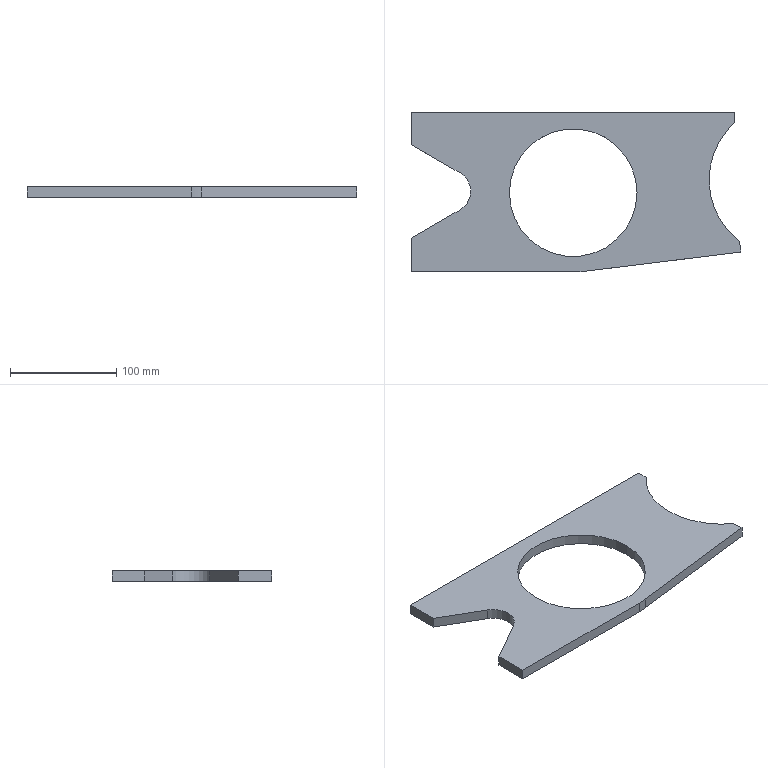Part | SolidWorks | features Extrusion 1 | 1 solid | 17 faces | box 309.8 x 150 x 10 mm | volume 282199 mm3 | plane 11 | cylinder 6 | commonest cylinder face diameters 120 x2 144.6 x2 40 x1 150 x1
STEP:
#1=CARTESIAN_POINT('',(-260.,-12.,10.));
#2=VERTEX_POINT('',#1);
#3=CARTESIAN_POINT('',(-140.,-12.,10.));
#4=VERTEX_POINT('',#3);
#5=CARTESIAN_POINT('',(-200.,-12.,10.));
#6=DIRECTION('',(0.,0.,1.));
#7=DIRECTION('',(1.,0.,0.));
#8=AXIS2_PLACEMENT_3D('',#5,#6,#7);
#9=CIRCLE('',#8,60.);
#10=EDGE_CURVE('',#2,#4,#9,.T.);
#11=ORIENTED_EDGE('',*,*,#10,.T.);
#12=CARTESIAN_POINT('',(-140.,-12.,0.));
#13=VERTEX_POINT('',#12);
#14=CARTESIAN_POINT('',(-140.,-12.,10.));
#15=DIRECTION('',(0.,0.,-1.));
#16=VECTOR('',#15,1000.);
#17=LINE('',#14,#16);
#18=EDGE_CURVE('',#4,#13,#17,.T.);
#19=ORIENTED_EDGE('',*,*,#18,.T.);
#20=CARTESIAN_POINT('',(-260.,-12.,0.));
#21=VERTEX_POINT('',#20);
#22=CARTESIAN_POINT('',(-200.,-12.,0.));
#23=DIRECTION('',(0.,0.,1.));
#24=DIRECTION('',(1.,0.,0.));
#25=AXIS2_PLACEMENT_3D('',#22,#23,#24);
#26=CIRCLE('',#25,60.);
#27=EDGE_CURVE('',#21,#13,#26,.T.);
#28=ORIENTED_EDGE('',*,*,#27,.F.);
#29=CARTESIAN_POINT('',(-260.,-12.,10.));
#30=DIRECTION('',(0.,0.,-1.));
#31=VECTOR('',#30,1000.);
#32=LINE('',#29,#31);
#33=EDGE_CURVE('',#2,#21,#32,.T.);
#34=ORIENTED_EDGE('',*,*,#33,.F.);
#35=EDGE_LOOP('',(#11,#19,#28,#34));
#36=FACE_OUTER_BOUND('',#35,.T.);
#37=CARTESIAN_POINT('',(-200.,-12.,10.));
#38=DIRECTION('',(0.,0.,-1.));
#39=DIRECTION('',(-1.,0.,0.));
#40=AXIS2_PLACEMENT_3D('',#37,#38,#39);
#41=CYLINDRICAL_SURFACE('',#40,60.);
#42=ADVANCED_FACE('',(#36),#41,.F.);
#43=CARTESIAN_POINT('',(-72.3,0.,10.));
#44=VERTEX_POINT('',#43);
#45=CARTESIAN_POINT('',(-48.3,53.8,10.));
#46=VERTEX_POINT('',#45);
#47=CARTESIAN_POINT('',(0.,0.,10.));
#48=DIRECTION('',(0.,0.,-1.));
#49=DIRECTION('',(1.,0.,0.));
#50=AXIS2_PLACEMENT_3D('',#47,#48,#49);
#51=CIRCLE('',#50,72.3);
#52=EDGE_CURVE('',#44,#46,#51,.T.);
#53=ORIENTED_EDGE('',*,*,#52,.F.);
#54=CARTESIAN_POINT('',(-72.3,0.,0.));
#55=VERTEX_POINT('',#54);
#56=CARTESIAN_POINT('',(-72.3,0.,10.));
#57=DIRECTION('',(0.,0.,-1.));
#58=VECTOR('',#57,1000.);
#59=LINE('',#56,#58);
#60=EDGE_CURVE('',#44,#55,#59,.T.);
#61=ORIENTED_EDGE('',*,*,#60,.T.);
#62=CARTESIAN_POINT('',(-48.3,53.8,0.));
#63=VERTEX_POINT('',#62);
#64=CARTESIAN_POINT('',(0.,0.,0.));
#65=DIRECTION('',(0.,0.,-1.));
#66=DIRECTION('',(1.,0.,0.));
#67=AXIS2_PLACEMENT_3D('',#64,#65,#66);
#68=CIRCLE('',#67,72.3);
#69=EDGE_CURVE('',#55,#63,#68,.T.);
#70=ORIENTED_EDGE('',*,*,#69,.T.);
#71=CARTESIAN_POINT('',(-48.3,53.8,10.));
#72=DIRECTION('',(0.,0.,-1.));
#73=VECTOR('',#72,1000.);
#74=LINE('',#71,#73);
#75=EDGE_CURVE('',#46,#63,#74,.T.);
#76=ORIENTED_EDGE('',*,*,#75,.F.);
#77=EDGE_LOOP('',(#53,#61,#70,#76));
#78=FACE_OUTER_BOUND('',#77,.T.);
#79=CARTESIAN_POINT('',(0.,0.,10.));
#80=DIRECTION('',(0.,0.,-1.));
#81=DIRECTION('',(-1.,0.,0.));
#82=AXIS2_PLACEMENT_3D('',#79,#80,#81);
#83=CYLINDRICAL_SURFACE('',#82,72.3);
#84=ADVANCED_FACE('',(#78),#83,.F.);
#85=CARTESIAN_POINT('',(-43.758,-57.555,10.));
#86=VERTEX_POINT('',#85);
#87=CARTESIAN_POINT('',(0.,0.,10.));
#88=DIRECTION('',(0.,0.,-1.));
#89=DIRECTION('',(1.,0.,0.));
#90=AXIS2_PLACEMENT_3D('',#87,#88,#89);
#91=CIRCLE('',#90,72.3);
#92=EDGE_CURVE('',#86,#44,#91,.T.);
#93=ORIENTED_EDGE('',*,*,#92,.T.);
#94=ORIENTED_EDGE('',*,*,#52,.T.);
#95=CARTESIAN_POINT('',(-48.3,63.7,10.));
#96=VERTEX_POINT('',#95);
#97=CARTESIAN_POINT('',(-48.3,63.7,10.));
#98=DIRECTION('',(0.,1.,0.));
#99=VECTOR('',#98,1000.);
#100=LINE('',#97,#99);
#101=EDGE_CURVE('',#46,#96,#100,.T.);
#102=ORIENTED_EDGE('',*,*,#101,.T.);
#103=CARTESIAN_POINT('',(-352.3,63.7,10.));
#104=VERTEX_POINT('',#103);
#105=CARTESIAN_POINT('',(-48.3,63.7,10.));
#106=DIRECTION('',(-1.,0.,0.));
#107=VECTOR('',#106,1000.);
#108=LINE('',#105,#107);
#109=EDGE_CURVE('',#96,#104,#108,.T.);
#110=ORIENTED_EDGE('',*,*,#109,.T.);
#111=CARTESIAN_POINT('',(-352.3,33.1,10.));
#112=VERTEX_POINT('',#111);
#113=CARTESIAN_POINT('',(-352.3,63.7,10.));
#114=DIRECTION('',(0.,-1.,0.));
#115=VECTOR('',#114,1000.);
#116=LINE('',#113,#115);
#117=EDGE_CURVE('',#104,#112,#116,.T.);
#118=ORIENTED_EDGE('',*,*,#117,.T.);
#119=CARTESIAN_POINT('',(-306.35,6.571,10.));
#120=VERTEX_POINT('',#119);
#121=CARTESIAN_POINT('',(-352.3,33.1,10.));
#122=DIRECTION('',(0.866,-0.5,0.));
#123=VECTOR('',#122,1000.);
#124=LINE('',#121,#123);
#125=EDGE_CURVE('',#112,#120,#124,.T.);
#126=ORIENTED_EDGE('',*,*,#125,.T.);
#127=CARTESIAN_POINT('',(-306.35,-28.071,10.));
#128=VERTEX_POINT('',#127);
#129=CARTESIAN_POINT('',(-316.35,-10.75,10.));
#130=DIRECTION('',(0.,0.,-1.));
#131=DIRECTION('',(1.,0.,0.));
#132=AXIS2_PLACEMENT_3D('',#129,#130,#131);
#133=CIRCLE('',#132,20.);
#134=EDGE_CURVE('',#120,#128,#133,.T.);
#135=ORIENTED_EDGE('',*,*,#134,.T.);
#136=CARTESIAN_POINT('',(-352.3,-54.6,10.));
#137=VERTEX_POINT('',#136);
#138=CARTESIAN_POINT('',(-306.35,-28.071,10.));
#139=DIRECTION('',(-0.866,-0.5,0.));
#140=VECTOR('',#139,1000.);
#141=LINE('',#138,#140);
#142=EDGE_CURVE('',#128,#137,#141,.T.);
#143=ORIENTED_EDGE('',*,*,#142,.T.);
#144=CARTESIAN_POINT('',(-352.3,-86.3,10.));
#145=VERTEX_POINT('',#144);
#146=CARTESIAN_POINT('',(-352.3,-54.6,10.));
#147=DIRECTION('',(0.,-1.,0.));
#148=VECTOR('',#147,1000.);
#149=LINE('',#146,#148);
#150=EDGE_CURVE('',#137,#145,#149,.T.);
#151=ORIENTED_EDGE('',*,*,#150,.T.);
#152=CARTESIAN_POINT('',(-197.758,-86.3,10.));
#153=VERTEX_POINT('',#152);
#154=CARTESIAN_POINT('',(-352.3,-86.3,10.));
#155=DIRECTION('',(1.,0.,0.));
#156=VECTOR('',#155,1000.);
#157=LINE('',#154,#156);
#158=EDGE_CURVE('',#145,#153,#157,.T.);
#159=ORIENTED_EDGE('',*,*,#158,.T.);
#160=CARTESIAN_POINT('',(-188.617,-85.741,10.));
#161=VERTEX_POINT('',#160);
#162=CARTESIAN_POINT('',(-197.758,-11.3,10.));
#163=DIRECTION('',(0.,0.,1.));
#164=DIRECTION('',(-1.,0.,0.));
#165=AXIS2_PLACEMENT_3D('',#162,#163,#164);
#166=CIRCLE('',#165,75.);
#167=EDGE_CURVE('',#153,#161,#166,.T.);
#168=ORIENTED_EDGE('',*,*,#167,.T.);
#169=CARTESIAN_POINT('',(-42.5,-67.8,10.));
#170=VERTEX_POINT('',#169);
#171=CARTESIAN_POINT('',(-188.617,-85.741,10.));
#172=DIRECTION('',(0.9925,0.1219,0.));
#173=VECTOR('',#172,1000.);
#174=LINE('',#171,#173);
#175=EDGE_CURVE('',#161,#170,#174,.T.);
#176=ORIENTED_EDGE('',*,*,#175,.T.);
#177=CARTESIAN_POINT('',(-42.5,-67.8,10.));
#178=DIRECTION('',(-0.1219,0.9925,0.));
#179=VECTOR('',#178,1000.);
#180=LINE('',#177,#179);
#181=EDGE_CURVE('',#170,#86,#180,.T.);
#182=ORIENTED_EDGE('',*,*,#181,.T.);
#183=EDGE_LOOP('',(#93,#94,#102,#110,#118,#126,#135,#143,#151,#159,#168,#176,#182));
#184=FACE_OUTER_BOUND('',#183,.T.);
#185=ORIENTED_EDGE('',*,*,#10,.F.);
#186=CARTESIAN_POINT('',(-200.,-12.,10.));
#187=DIRECTION('',(0.,0.,1.));
#188=DIRECTION('',(1.,0.,0.));
#189=AXIS2_PLACEMENT_3D('',#186,#187,#188);
#190=CIRCLE('',#189,60.);
#191=EDGE_CURVE('',#4,#2,#190,.T.);
#192=ORIENTED_EDGE('',*,*,#191,.F.);
#193=EDGE_LOOP('',(#185,#192));
#194=FACE_BOUND('',#193,.T.);
#195=CARTESIAN_POINT('',(0.,0.,10.));
#196=DIRECTION('',(0.,0.,1.));
#197=DIRECTION('',(1.,0.,0.));
#198=AXIS2_PLACEMENT_3D('',#195,#196,#197);
#199=PLANE('',#198);
#200=ADVANCED_FACE('',(#184,#194),#199,.T.);
#201=CARTESIAN_POINT('',(-43.758,-57.555,0.));
#202=VERTEX_POINT('',#201);
#203=CARTESIAN_POINT('',(0.,0.,0.));
#204=DIRECTION('',(0.,0.,-1.));
#205=DIRECTION('',(1.,0.,0.));
#206=AXIS2_PLACEMENT_3D('',#203,#204,#205);
#207=CIRCLE('',#206,72.3);
#208=EDGE_CURVE('',#202,#55,#207,.T.);
#209=ORIENTED_EDGE('',*,*,#208,.F.);
#210=CARTESIAN_POINT('',(-42.5,-67.8,0.));
#211=VERTEX_POINT('',#210);
#212=CARTESIAN_POINT('',(-42.5,-67.8,0.));
#213=DIRECTION('',(-0.1219,0.9925,0.));
#214=VECTOR('',#213,1000.);
#215=LINE('',#212,#214);
#216=EDGE_CURVE('',#211,#202,#215,.T.);
#217=ORIENTED_EDGE('',*,*,#216,.F.);
#218=CARTESIAN_POINT('',(-188.617,-85.741,0.));
#219=VERTEX_POINT('',#218);
#220=CARTESIAN_POINT('',(-188.617,-85.741,0.));
#221=DIRECTION('',(0.9925,0.1219,0.));
#222=VECTOR('',#221,1000.);
#223=LINE('',#220,#222);
#224=EDGE_CURVE('',#219,#211,#223,.T.);
#225=ORIENTED_EDGE('',*,*,#224,.F.);
#226=CARTESIAN_POINT('',(-197.758,-86.3,0.));
#227=VERTEX_POINT('',#226);
#228=CARTESIAN_POINT('',(-197.758,-11.3,0.));
#229=DIRECTION('',(0.,0.,1.));
#230=DIRECTION('',(-1.,0.,0.));
#231=AXIS2_PLACEMENT_3D('',#228,#229,#230);
#232=CIRCLE('',#231,75.);
#233=EDGE_CURVE('',#227,#219,#232,.T.);
#234=ORIENTED_EDGE('',*,*,#233,.F.);
#235=CARTESIAN_POINT('',(-352.3,-86.3,0.));
#236=VERTEX_POINT('',#235);
#237=CARTESIAN_POINT('',(-352.3,-86.3,0.));
#238=DIRECTION('',(1.,0.,0.));
#239=VECTOR('',#238,1000.);
#240=LINE('',#237,#239);
#241=EDGE_CURVE('',#236,#227,#240,.T.);
#242=ORIENTED_EDGE('',*,*,#241,.F.);
#243=CARTESIAN_POINT('',(-352.3,-54.6,0.));
#244=VERTEX_POINT('',#243);
#245=CARTESIAN_POINT('',(-352.3,-54.6,0.));
#246=DIRECTION('',(0.,-1.,0.));
#247=VECTOR('',#246,1000.);
#248=LINE('',#245,#247);
#249=EDGE_CURVE('',#244,#236,#248,.T.);
#250=ORIENTED_EDGE('',*,*,#249,.F.);
#251=CARTESIAN_POINT('',(-306.35,-28.071,0.));
#252=VERTEX_POINT('',#251);
#253=CARTESIAN_POINT('',(-306.35,-28.071,0.));
#254=DIRECTION('',(-0.866,-0.5,0.));
#255=VECTOR('',#254,1000.);
#256=LINE('',#253,#255);
#257=EDGE_CURVE('',#252,#244,#256,.T.);
#258=ORIENTED_EDGE('',*,*,#257,.F.);
#259=CARTESIAN_POINT('',(-306.35,6.571,0.));
#260=VERTEX_POINT('',#259);
#261=CARTESIAN_POINT('',(-316.35,-10.75,0.));
#262=DIRECTION('',(0.,0.,-1.));
#263=DIRECTION('',(1.,0.,0.));
#264=AXIS2_PLACEMENT_3D('',#261,#262,#263);
#265=CIRCLE('',#264,20.);
#266=EDGE_CURVE('',#260,#252,#265,.T.);
#267=ORIENTED_EDGE('',*,*,#266,.F.);
#268=CARTESIAN_POINT('',(-352.3,33.1,0.));
#269=VERTEX_POINT('',#268);
#270=CARTESIAN_POINT('',(-352.3,33.1,0.));
#271=DIRECTION('',(0.866,-0.5,0.));
#272=VECTOR('',#271,1000.);
#273=LINE('',#270,#272);
#274=EDGE_CURVE('',#269,#260,#273,.T.);
#275=ORIENTED_EDGE('',*,*,#274,.F.);
#276=CARTESIAN_POINT('',(-352.3,63.7,0.));
#277=VERTEX_POINT('',#276);
#278=CARTESIAN_POINT('',(-352.3,63.7,0.));
#279=DIRECTION('',(0.,-1.,0.));
#280=VECTOR('',#279,1000.);
#281=LINE('',#278,#280);
#282=EDGE_CURVE('',#277,#269,#281,.T.);
#283=ORIENTED_EDGE('',*,*,#282,.F.);
#284=CARTESIAN_POINT('',(-48.3,63.7,0.));
#285=VERTEX_POINT('',#284);
#286=CARTESIAN_POINT('',(-48.3,63.7,0.));
#287=DIRECTION('',(-1.,0.,0.));
#288=VECTOR('',#287,1000.);
#289=LINE('',#286,#288);
#290=EDGE_CURVE('',#285,#277,#289,.T.);
#291=ORIENTED_EDGE('',*,*,#290,.F.);
#292=CARTESIAN_POINT('',(-48.3,63.7,0.));
#293=DIRECTION('',(0.,1.,0.));
#294=VECTOR('',#293,1000.);
#295=LINE('',#292,#294);
#296=EDGE_CURVE('',#63,#285,#295,.T.);
#297=ORIENTED_EDGE('',*,*,#296,.F.);
#298=ORIENTED_EDGE('',*,*,#69,.F.);
#299=EDGE_LOOP('',(#209,#217,#225,#234,#242,#250,#258,#267,#275,#283,#291,#297,#298));
#300=FACE_OUTER_BOUND('',#299,.T.);
#301=ORIENTED_EDGE('',*,*,#27,.T.);
#302=CARTESIAN_POINT('',(-200.,-12.,0.));
#303=DIRECTION('',(0.,0.,1.));
#304=DIRECTION('',(1.,0.,0.));
#305=AXIS2_PLACEMENT_3D('',#302,#303,#304);
#306=CIRCLE('',#305,60.);
#307=EDGE_CURVE('',#13,#21,#306,.T.);
#308=ORIENTED_EDGE('',*,*,#307,.T.);
#309=EDGE_LOOP('',(#301,#308));
#310=FACE_BOUND('',#309,.T.);
#311=CARTESIAN_POINT('',(0.,0.,0.));
#312=DIRECTION('',(0.,0.,1.));
#313=DIRECTION('',(1.,0.,0.));
#314=AXIS2_PLACEMENT_3D('',#311,#312,#313);
#315=PLANE('',#314);
#316=ADVANCED_FACE('',(#300,#310),#315,.F.);
#317=ORIENTED_EDGE('',*,*,#60,.F.);
#318=ORIENTED_EDGE('',*,*,#92,.F.);
#319=CARTESIAN_POINT('',(-43.758,-57.555,10.));
#320=DIRECTION('',(0.,0.,-1.));
#321=VECTOR('',#320,1000.);
#322=LINE('',#319,#321);
#323=EDGE_CURVE('',#86,#202,#322,.T.);
#324=ORIENTED_EDGE('',*,*,#323,.T.);
#325=ORIENTED_EDGE('',*,*,#208,.T.);
#326=EDGE_LOOP('',(#317,#318,#324,#325));
#327=FACE_OUTER_BOUND('',#326,.T.);
#328=CARTESIAN_POINT('',(0.,0.,10.));
#329=DIRECTION('',(0.,0.,-1.));
#330=DIRECTION('',(-1.,0.,0.));
#331=AXIS2_PLACEMENT_3D('',#328,#329,#330);
#332=CYLINDRICAL_SURFACE('',#331,72.3);
#333=ADVANCED_FACE('',(#327),#332,.F.);
#334=ORIENTED_EDGE('',*,*,#296,.T.);
#335=CARTESIAN_POINT('',(-48.3,63.7,10.));
#336=DIRECTION('',(0.,0.,-1.));
#337=VECTOR('',#336,1000.);
#338=LINE('',#335,#337);
#339=EDGE_CURVE('',#96,#285,#338,.T.);
#340=ORIENTED_EDGE('',*,*,#339,.F.);
#341=ORIENTED_EDGE('',*,*,#101,.F.);
#342=ORIENTED_EDGE('',*,*,#75,.T.);
#343=EDGE_LOOP('',(#334,#340,#341,#342));
#344=FACE_OUTER_BOUND('',#343,.T.);
#345=CARTESIAN_POINT('',(-48.3,63.7,10.));
#346=DIRECTION('',(-1.,0.,0.));
#347=DIRECTION('',(0.,0.,1.));
#348=AXIS2_PLACEMENT_3D('',#345,#346,#347);
#349=PLANE('',#348);
#350=ADVANCED_FACE('',(#344),#349,.F.);
#351=ORIENTED_EDGE('',*,*,#290,.T.);
#352=CARTESIAN_POINT('',(-352.3,63.7,10.));
#353=DIRECTION('',(0.,0.,-1.));
#354=VECTOR('',#353,1000.);
#355=LINE('',#352,#354);
#356=EDGE_CURVE('',#104,#277,#355,.T.);
#357=ORIENTED_EDGE('',*,*,#356,.F.);
#358=ORIENTED_EDGE('',*,*,#109,.F.);
#359=ORIENTED_EDGE('',*,*,#339,.T.);
#360=EDGE_LOOP('',(#351,#357,#358,#359));
#361=FACE_OUTER_BOUND('',#360,.T.);
#362=CARTESIAN_POINT('',(-48.3,63.7,10.));
#363=DIRECTION('',(0.,-1.,0.));
#364=DIRECTION('',(1.,0.,0.));
#365=AXIS2_PLACEMENT_3D('',#362,#363,#364);
#366=PLANE('',#365);
#367=ADVANCED_FACE('',(#361),#366,.F.);
#368=ORIENTED_EDGE('',*,*,#282,.T.);
#369=CARTESIAN_POINT('',(-352.3,33.1,10.));
#370=DIRECTION('',(0.,0.,-1.));
#371=VECTOR('',#370,1000.);
#372=LINE('',#369,#371);
#373=EDGE_CURVE('',#112,#269,#372,.T.);
#374=ORIENTED_EDGE('',*,*,#373,.F.);
#375=ORIENTED_EDGE('',*,*,#117,.F.);
#376=ORIENTED_EDGE('',*,*,#356,.T.);
#377=EDGE_LOOP('',(#368,#374,#375,#376));
#378=FACE_OUTER_BOUND('',#377,.T.);
#379=CARTESIAN_POINT('',(-352.3,63.7,10.));
#380=DIRECTION('',(1.,0.,0.));
#381=DIRECTION('',(0.,0.,-1.));
#382=AXIS2_PLACEMENT_3D('',#379,#380,#381);
#383=PLANE('',#382);
#384=ADVANCED_FACE('',(#378),#383,.F.);
#385=ORIENTED_EDGE('',*,*,#274,.T.);
#386=CARTESIAN_POINT('',(-306.35,6.571,10.));
#387=DIRECTION('',(0.,0.,-1.));
#388=VECTOR('',#387,1000.);
#389=LINE('',#386,#388);
#390=EDGE_CURVE('',#120,#260,#389,.T.);
#391=ORIENTED_EDGE('',*,*,#390,.F.);
#392=ORIENTED_EDGE('',*,*,#125,.F.);
#393=ORIENTED_EDGE('',*,*,#373,.T.);
#394=EDGE_LOOP('',(#385,#391,#392,#393));
#395=FACE_OUTER_BOUND('',#394,.T.);
#396=CARTESIAN_POINT('',(-352.3,33.1,10.));
#397=DIRECTION('',(0.5,0.866,0.));
#398=DIRECTION('',(-0.866,0.5,0.));
#399=AXIS2_PLACEMENT_3D('',#396,#397,#398);
#400=PLANE('',#399);
#401=ADVANCED_FACE('',(#395),#400,.F.);
#402=ORIENTED_EDGE('',*,*,#266,.T.);
#403=CARTESIAN_POINT('',(-306.35,-28.071,10.));
#404=DIRECTION('',(0.,0.,-1.));
#405=VECTOR('',#404,1000.);
#406=LINE('',#403,#405);
#407=EDGE_CURVE('',#128,#252,#406,.T.);
#408=ORIENTED_EDGE('',*,*,#407,.F.);
#409=ORIENTED_EDGE('',*,*,#134,.F.);
#410=ORIENTED_EDGE('',*,*,#390,.T.);
#411=EDGE_LOOP('',(#402,#408,#409,#410));
#412=FACE_OUTER_BOUND('',#411,.T.);
#413=CARTESIAN_POINT('',(-316.35,-10.75,10.));
#414=DIRECTION('',(0.,0.,-1.));
#415=DIRECTION('',(-1.,0.,0.));
#416=AXIS2_PLACEMENT_3D('',#413,#414,#415);
#417=CYLINDRICAL_SURFACE('',#416,20.);
#418=ADVANCED_FACE('',(#412),#417,.F.);
#419=ORIENTED_EDGE('',*,*,#257,.T.);
#420=CARTESIAN_POINT('',(-352.3,-54.6,10.));
#421=DIRECTION('',(0.,0.,-1.));
#422=VECTOR('',#421,1000.);
#423=LINE('',#420,#422);
#424=EDGE_CURVE('',#137,#244,#423,.T.);
#425=ORIENTED_EDGE('',*,*,#424,.F.);
#426=ORIENTED_EDGE('',*,*,#142,.F.);
#427=ORIENTED_EDGE('',*,*,#407,.T.);
#428=EDGE_LOOP('',(#419,#425,#426,#427));
#429=FACE_OUTER_BOUND('',#428,.T.);
#430=CARTESIAN_POINT('',(-306.35,-28.071,10.));
#431=DIRECTION('',(0.5,-0.866,0.));
#432=DIRECTION('',(0.866,0.5,0.));
#433=AXIS2_PLACEMENT_3D('',#430,#431,#432);
#434=PLANE('',#433);
#435=ADVANCED_FACE('',(#429),#434,.F.);
#436=ORIENTED_EDGE('',*,*,#249,.T.);
#437=CARTESIAN_POINT('',(-352.3,-86.3,10.));
#438=DIRECTION('',(0.,0.,-1.));
#439=VECTOR('',#438,1000.);
#440=LINE('',#437,#439);
#441=EDGE_CURVE('',#145,#236,#440,.T.);
#442=ORIENTED_EDGE('',*,*,#441,.F.);
#443=ORIENTED_EDGE('',*,*,#150,.F.);
#444=ORIENTED_EDGE('',*,*,#424,.T.);
#445=EDGE_LOOP('',(#436,#442,#443,#444));
#446=FACE_OUTER_BOUND('',#445,.T.);
#447=CARTESIAN_POINT('',(-352.3,-54.6,10.));
#448=DIRECTION('',(1.,0.,0.));
#449=DIRECTION('',(0.,0.,-1.));
#450=AXIS2_PLACEMENT_3D('',#447,#448,#449);
#451=PLANE('',#450);
#452=ADVANCED_FACE('',(#446),#451,.F.);
#453=ORIENTED_EDGE('',*,*,#241,.T.);
#454=CARTESIAN_POINT('',(-197.758,-86.3,10.));
#455=DIRECTION('',(0.,0.,-1.));
#456=VECTOR('',#455,1000.);
#457=LINE('',#454,#456);
#458=EDGE_CURVE('',#153,#227,#457,.T.);
#459=ORIENTED_EDGE('',*,*,#458,.F.);
#460=ORIENTED_EDGE('',*,*,#158,.F.);
#461=ORIENTED_EDGE('',*,*,#441,.T.);
#462=EDGE_LOOP('',(#453,#459,#460,#461));
#463=FACE_OUTER_BOUND('',#462,.T.);
#464=CARTESIAN_POINT('',(-352.3,-86.3,10.));
#465=DIRECTION('',(0.,1.,0.));
#466=DIRECTION('',(0.,0.,1.));
#467=AXIS2_PLACEMENT_3D('',#464,#465,#466);
#468=PLANE('',#467);
#469=ADVANCED_FACE('',(#463),#468,.F.);
#470=ORIENTED_EDGE('',*,*,#233,.T.);
#471=CARTESIAN_POINT('',(-188.617,-85.741,10.));
#472=DIRECTION('',(0.,0.,-1.));
#473=VECTOR('',#472,1000.);
#474=LINE('',#471,#473);
#475=EDGE_CURVE('',#161,#219,#474,.T.);
#476=ORIENTED_EDGE('',*,*,#475,.F.);
#477=ORIENTED_EDGE('',*,*,#167,.F.);
#478=ORIENTED_EDGE('',*,*,#458,.T.);
#479=EDGE_LOOP('',(#470,#476,#477,#478));
#480=FACE_OUTER_BOUND('',#479,.T.);
#481=CARTESIAN_POINT('',(-197.758,-11.3,10.));
#482=DIRECTION('',(0.,0.,-1.));
#483=DIRECTION('',(-1.,0.,0.));
#484=AXIS2_PLACEMENT_3D('',#481,#482,#483);
#485=CYLINDRICAL_SURFACE('',#484,75.);
#486=ADVANCED_FACE('',(#480),#485,.T.);
#487=ORIENTED_EDGE('',*,*,#224,.T.);
#488=CARTESIAN_POINT('',(-42.5,-67.8,10.));
#489=DIRECTION('',(0.,0.,-1.));
#490=VECTOR('',#489,1000.);
#491=LINE('',#488,#490);
#492=EDGE_CURVE('',#170,#211,#491,.T.);
#493=ORIENTED_EDGE('',*,*,#492,.F.);
#494=ORIENTED_EDGE('',*,*,#175,.F.);
#495=ORIENTED_EDGE('',*,*,#475,.T.);
#496=EDGE_LOOP('',(#487,#493,#494,#495));
#497=FACE_OUTER_BOUND('',#496,.T.);
#498=CARTESIAN_POINT('',(-188.617,-85.741,10.));
#499=DIRECTION('',(-0.1219,0.9925,0.));
#500=DIRECTION('',(-0.9925,-0.1219,0.));
#501=AXIS2_PLACEMENT_3D('',#498,#499,#500);
#502=PLANE('',#501);
#503=ADVANCED_FACE('',(#497),#502,.F.);
#504=ORIENTED_EDGE('',*,*,#216,.T.);
#505=ORIENTED_EDGE('',*,*,#323,.F.);
#506=ORIENTED_EDGE('',*,*,#181,.F.);
#507=ORIENTED_EDGE('',*,*,#492,.T.);
#508=EDGE_LOOP('',(#504,#505,#506,#507));
#509=FACE_OUTER_BOUND('',#508,.T.);
#510=CARTESIAN_POINT('',(-42.5,-67.8,10.));
#511=DIRECTION('',(-0.9925,-0.1219,0.));
#512=DIRECTION('',(0.1219,-0.9925,0.));
#513=AXIS2_PLACEMENT_3D('',#510,#511,#512);
#514=PLANE('',#513);
#515=ADVANCED_FACE('',(#509),#514,.F.);
#516=ORIENTED_EDGE('',*,*,#18,.F.);
#517=ORIENTED_EDGE('',*,*,#191,.T.);
#518=ORIENTED_EDGE('',*,*,#33,.T.);
#519=ORIENTED_EDGE('',*,*,#307,.F.);
#520=EDGE_LOOP('',(#516,#517,#518,#519));
#521=FACE_OUTER_BOUND('',#520,.T.);
#522=CARTESIAN_POINT('',(-200.,-12.,10.));
#523=DIRECTION('',(0.,0.,-1.));
#524=DIRECTION('',(-1.,0.,0.));
#525=AXIS2_PLACEMENT_3D('',#522,#523,#524);
#526=CYLINDRICAL_SURFACE('',#525,60.);
#527=ADVANCED_FACE('',(#521),#526,.F.);
#528=CLOSED_SHELL('',(#42,#84,#200,#316,#333,#350,#367,#384,#401,#418,#435,#452,#469,#486,#503,#515,#527));
#529=MANIFOLD_SOLID_BREP('',#528);
#530=CARTESIAN_POINT('',(0.,0.,0.));
#531=DIRECTION('',(0.,0.,1.));
#532=DIRECTION('',(1.,0.,0.));
#533=AXIS2_PLACEMENT_3D('',#530,#531,#532);
#534=(LENGTH_UNIT()NAMED_UNIT(*)SI_UNIT(.MILLI.,.METRE.));
#535=UNCERTAINTY_MEASURE_WITH_UNIT(LENGTH_MEASURE(0.00001),#534,'','');
#536=(NAMED_UNIT(*)PLANE_ANGLE_UNIT()SI_UNIT($,.RADIAN.));
#537=(NAMED_UNIT(*)SI_UNIT($,.STERADIAN.)SOLID_ANGLE_UNIT());
#538=(GEOMETRIC_REPRESENTATION_CONTEXT(3)GLOBAL_UNCERTAINTY_ASSIGNED_CONTEXT((#535))GLOBAL_UNIT_ASSIGNED_CONTEXT((#534,#536,#537))REPRESENTATION_CONTEXT('',''));
#539=ADVANCED_BREP_SHAPE_REPRESENTATION('',(#529,#533),#538);